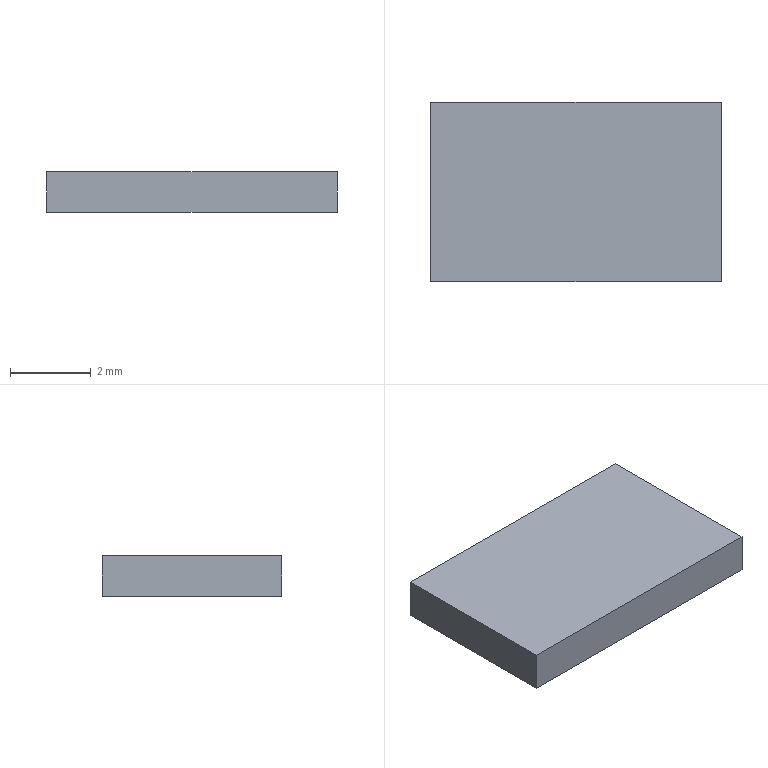Part | Creo | 1 solid | 6 faces | box 7.175 x 4.435 x 1 mm | volume 31.821 mm3 | plane 6
STEP:
#1=CARTESIAN_POINT('',(0.,0.,0.));
#2=DIRECTION('',(0.,0.,1.));
#3=DIRECTION('',(1.,0.,0.));
#4=AXIS2_PLACEMENT_3D('',#1,#2,#3);
#5=CARTESIAN_POINT('',(-3.675,-2.335,0.));
#6=VERTEX_POINT('',#5);
#7=CARTESIAN_POINT('',(3.5,-2.335,0.));
#8=VERTEX_POINT('',#7);
#9=CARTESIAN_POINT('',(-3.675,-2.335,0.));
#10=DIRECTION('',(1.,0.,0.));
#11=VECTOR('',#10,7.175);
#12=LINE('',#9,#11);
#13=EDGE_CURVE('',#6,#8,#12,.T.);
#14=ORIENTED_EDGE('',*,*,#13,.T.);
#15=CARTESIAN_POINT('',(3.5,2.1,0.));
#16=VERTEX_POINT('',#15);
#17=CARTESIAN_POINT('',(3.5,-2.335,0.));
#18=DIRECTION('',(0.,1.,0.));
#19=VECTOR('',#18,4.435);
#20=LINE('',#17,#19);
#21=EDGE_CURVE('',#8,#16,#20,.T.);
#22=ORIENTED_EDGE('',*,*,#21,.T.);
#23=CARTESIAN_POINT('',(-3.675,2.1,0.));
#24=VERTEX_POINT('',#23);
#25=CARTESIAN_POINT('',(3.5,2.1,0.));
#26=DIRECTION('',(-1.,0.,0.));
#27=VECTOR('',#26,7.175);
#28=LINE('',#25,#27);
#29=EDGE_CURVE('',#16,#24,#28,.T.);
#30=ORIENTED_EDGE('',*,*,#29,.T.);
#31=CARTESIAN_POINT('',(-3.675,2.1,0.));
#32=DIRECTION('',(0.,-1.,0.));
#33=VECTOR('',#32,4.435);
#34=LINE('',#31,#33);
#35=EDGE_CURVE('',#24,#6,#34,.T.);
#36=ORIENTED_EDGE('',*,*,#35,.T.);
#37=EDGE_LOOP('',(#14,#22,#30,#36));
#38=FACE_OUTER_BOUND('',#37,.F.);
#39=CARTESIAN_POINT('',(0.,0.,0.));
#40=DIRECTION('',(0.,0.,1.));
#41=DIRECTION('',(1.,0.,0.));
#42=AXIS2_PLACEMENT_3D('',#39,#40,#41);
#43=PLANE('',#42);
#44=ADVANCED_FACE('',(#38),#43,.F.);
#45=ORIENTED_EDGE('',*,*,#13,.F.);
#46=CARTESIAN_POINT('',(-3.675,-2.335,1.));
#47=VERTEX_POINT('',#46);
#48=CARTESIAN_POINT('',(-3.675,-2.335,0.));
#49=DIRECTION('',(0.,0.,1.));
#50=VECTOR('',#49,1.);
#51=LINE('',#48,#50);
#52=EDGE_CURVE('',#6,#47,#51,.T.);
#53=ORIENTED_EDGE('',*,*,#52,.T.);
#54=CARTESIAN_POINT('',(3.5,-2.335,1.));
#55=VERTEX_POINT('',#54);
#56=CARTESIAN_POINT('',(-3.675,-2.335,1.));
#57=DIRECTION('',(1.,0.,0.));
#58=VECTOR('',#57,7.175);
#59=LINE('',#56,#58);
#60=EDGE_CURVE('',#47,#55,#59,.T.);
#61=ORIENTED_EDGE('',*,*,#60,.T.);
#62=CARTESIAN_POINT('',(3.5,-2.335,0.));
#63=DIRECTION('',(0.,0.,1.));
#64=VECTOR('',#63,1.);
#65=LINE('',#62,#64);
#66=EDGE_CURVE('',#8,#55,#65,.T.);
#67=ORIENTED_EDGE('',*,*,#66,.F.);
#68=EDGE_LOOP('',(#45,#53,#61,#67));
#69=FACE_OUTER_BOUND('',#68,.F.);
#70=CARTESIAN_POINT('',(-3.675,-2.335,0.));
#71=DIRECTION('',(0.,-1.,0.));
#72=DIRECTION('',(1.,0.,0.));
#73=AXIS2_PLACEMENT_3D('',#70,#71,#72);
#74=PLANE('',#73);
#75=ADVANCED_FACE('',(#69),#74,.T.);
#76=ORIENTED_EDGE('',*,*,#35,.F.);
#77=CARTESIAN_POINT('',(-3.675,2.1,1.));
#78=VERTEX_POINT('',#77);
#79=CARTESIAN_POINT('',(-3.675,2.1,0.));
#80=DIRECTION('',(0.,0.,1.));
#81=VECTOR('',#80,1.);
#82=LINE('',#79,#81);
#83=EDGE_CURVE('',#24,#78,#82,.T.);
#84=ORIENTED_EDGE('',*,*,#83,.T.);
#85=CARTESIAN_POINT('',(-3.675,2.1,1.));
#86=DIRECTION('',(0.,-1.,0.));
#87=VECTOR('',#86,4.435);
#88=LINE('',#85,#87);
#89=EDGE_CURVE('',#78,#47,#88,.T.);
#90=ORIENTED_EDGE('',*,*,#89,.T.);
#91=ORIENTED_EDGE('',*,*,#52,.F.);
#92=EDGE_LOOP('',(#76,#84,#90,#91));
#93=FACE_OUTER_BOUND('',#92,.F.);
#94=CARTESIAN_POINT('',(-3.675,2.1,0.));
#95=DIRECTION('',(-1.,0.,0.));
#96=DIRECTION('',(0.,-1.,0.));
#97=AXIS2_PLACEMENT_3D('',#94,#95,#96);
#98=PLANE('',#97);
#99=ADVANCED_FACE('',(#93),#98,.T.);
#100=ORIENTED_EDGE('',*,*,#29,.F.);
#101=CARTESIAN_POINT('',(3.5,2.1,1.));
#102=VERTEX_POINT('',#101);
#103=CARTESIAN_POINT('',(3.5,2.1,0.));
#104=DIRECTION('',(0.,0.,1.));
#105=VECTOR('',#104,1.);
#106=LINE('',#103,#105);
#107=EDGE_CURVE('',#16,#102,#106,.T.);
#108=ORIENTED_EDGE('',*,*,#107,.T.);
#109=CARTESIAN_POINT('',(3.5,2.1,1.));
#110=DIRECTION('',(-1.,0.,0.));
#111=VECTOR('',#110,7.175);
#112=LINE('',#109,#111);
#113=EDGE_CURVE('',#102,#78,#112,.T.);
#114=ORIENTED_EDGE('',*,*,#113,.T.);
#115=ORIENTED_EDGE('',*,*,#83,.F.);
#116=EDGE_LOOP('',(#100,#108,#114,#115));
#117=FACE_OUTER_BOUND('',#116,.F.);
#118=CARTESIAN_POINT('',(3.5,2.1,0.));
#119=DIRECTION('',(0.,1.,0.));
#120=DIRECTION('',(-1.,0.,0.));
#121=AXIS2_PLACEMENT_3D('',#118,#119,#120);
#122=PLANE('',#121);
#123=ADVANCED_FACE('',(#117),#122,.T.);
#124=ORIENTED_EDGE('',*,*,#21,.F.);
#125=ORIENTED_EDGE('',*,*,#66,.T.);
#126=CARTESIAN_POINT('',(3.5,-2.335,1.));
#127=DIRECTION('',(0.,1.,0.));
#128=VECTOR('',#127,4.435);
#129=LINE('',#126,#128);
#130=EDGE_CURVE('',#55,#102,#129,.T.);
#131=ORIENTED_EDGE('',*,*,#130,.T.);
#132=ORIENTED_EDGE('',*,*,#107,.F.);
#133=EDGE_LOOP('',(#124,#125,#131,#132));
#134=FACE_OUTER_BOUND('',#133,.F.);
#135=CARTESIAN_POINT('',(3.5,-2.335,0.));
#136=DIRECTION('',(1.,0.,0.));
#137=DIRECTION('',(0.,1.,0.));
#138=AXIS2_PLACEMENT_3D('',#135,#136,#137);
#139=PLANE('',#138);
#140=ADVANCED_FACE('',(#134),#139,.T.);
#141=ORIENTED_EDGE('',*,*,#60,.F.);
#142=ORIENTED_EDGE('',*,*,#89,.F.);
#143=ORIENTED_EDGE('',*,*,#113,.F.);
#144=ORIENTED_EDGE('',*,*,#130,.F.);
#145=EDGE_LOOP('',(#141,#142,#143,#144));
#146=FACE_OUTER_BOUND('',#145,.F.);
#147=CARTESIAN_POINT('',(0.,0.,1.));
#148=DIRECTION('',(0.,0.,1.));
#149=DIRECTION('',(1.,0.,0.));
#150=AXIS2_PLACEMENT_3D('',#147,#148,#149);
#151=PLANE('',#150);
#152=ADVANCED_FACE('',(#146),#151,.T.);
#153=CLOSED_SHELL('',(#44,#75,#99,#123,#140,#152));
#154=MANIFOLD_SOLID_BREP('',#153);
#155=(LENGTH_UNIT()NAMED_UNIT(*)SI_UNIT(.MILLI.,.METRE.));
#156=UNCERTAINTY_MEASURE_WITH_UNIT(LENGTH_MEASURE(0.0008494),#155,'','');
#157=(NAMED_UNIT(*)PLANE_ANGLE_UNIT()SI_UNIT($,.RADIAN.));
#158=PLANE_ANGLE_MEASURE_WITH_UNIT(PLANE_ANGLE_MEASURE(0.01745),#157);
#159=(CONVERSION_BASED_UNIT('DEGREE',#158)NAMED_UNIT(*)PLANE_ANGLE_UNIT());
#160=(NAMED_UNIT(*)SI_UNIT($,.STERADIAN.)SOLID_ANGLE_UNIT());
#161=(GEOMETRIC_REPRESENTATION_CONTEXT(3)GLOBAL_UNCERTAINTY_ASSIGNED_CONTEXT((#156))GLOBAL_UNIT_ASSIGNED_CONTEXT((#155,#159,#160))REPRESENTATION_CONTEXT('',''));
#162=ADVANCED_BREP_SHAPE_REPRESENTATION('',(#4,#154),#161);